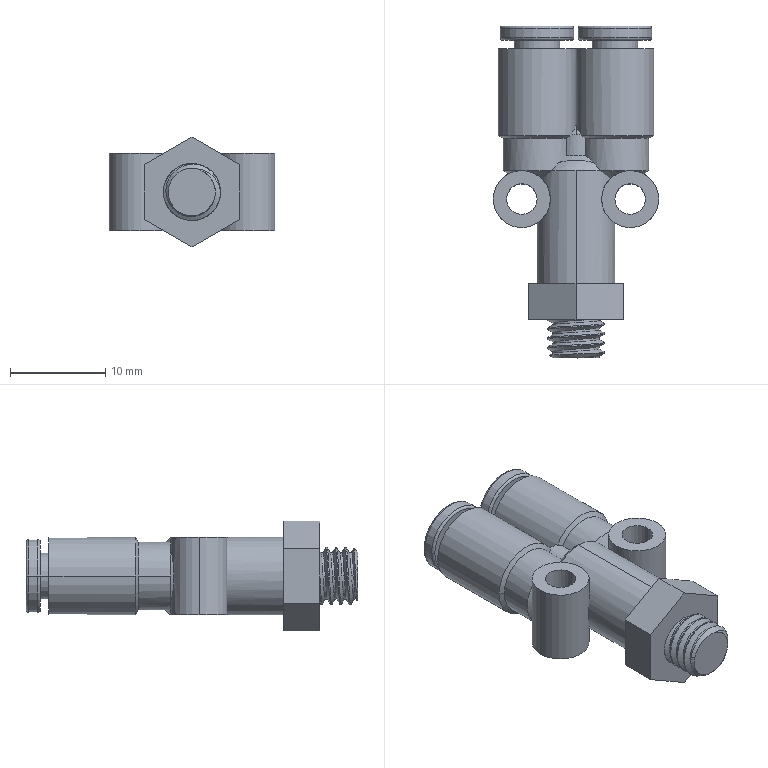Part | SolidWorks | 4 solids | 110 faces | box 17.4 x 34.9 x 11.547 mm | volume 2470 mm3 | cylinder 54 | plane 24 | cone 14 | torus 12 | sphere 4 | spline 2 | commonest cylinder face diameters 6 x12 4.918 x10 4.8 x8 3.2 x4 4 x4 7.15 x4